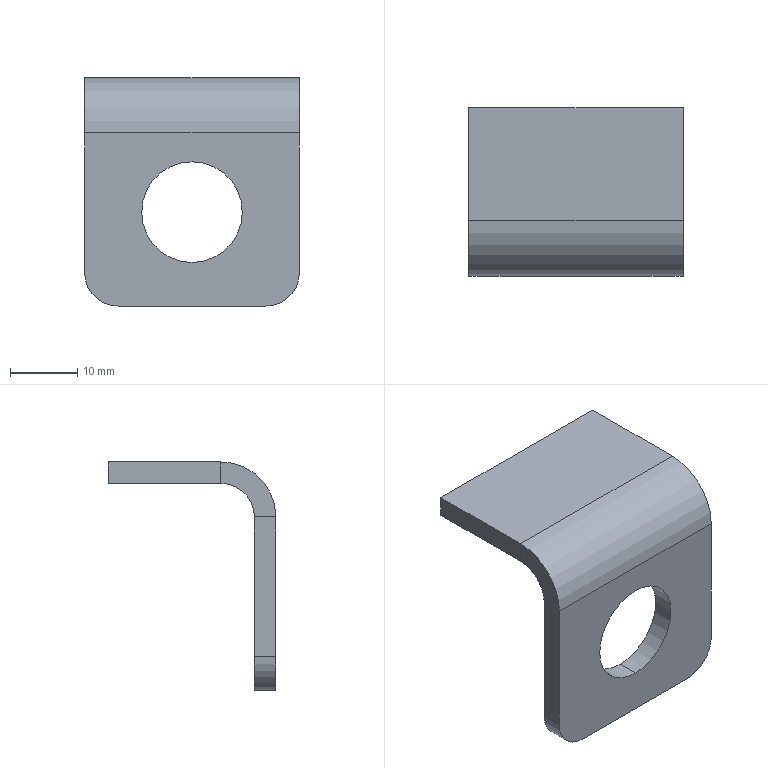Part | SolidWorks | features Fillet 1, FlatPattern 1, ICE 1, SMBaseFlange 1, SheetMetal 1 | 1 solid | 18 faces | box 32 x 25 x 34 mm | volume 4824 mm3 | plane 12 | cylinder 6 | commonest cylinder face diameters 10 x3 15 x2 16.4 x1
STEP:
#1=CARTESIAN_POINT('',(0.,3.2,-12.5));
#2=VERTEX_POINT('',#1);
#3=CARTESIAN_POINT('',(0.,3.2,-27.5));
#4=VERTEX_POINT('',#3);
#5=CARTESIAN_POINT('',(0.,3.2,-20.));
#6=DIRECTION('',(0.,-1.,0.));
#7=DIRECTION('',(0.,0.,-1.));
#8=AXIS2_PLACEMENT_3D('',#5,#6,#7);
#9=CIRCLE('',#8,7.5);
#10=EDGE_CURVE('',#2,#4,#9,.T.);
#11=ORIENTED_EDGE('',*,*,#10,.F.);
#12=CARTESIAN_POINT('',(0.,0.,-12.5));
#13=VERTEX_POINT('',#12);
#14=CARTESIAN_POINT('',(0.,25.,-12.5));
#15=DIRECTION('',(0.,-1.,0.));
#16=VECTOR('',#15,1000.);
#17=LINE('',#14,#16);
#18=EDGE_CURVE('',#2,#13,#17,.T.);
#19=ORIENTED_EDGE('',*,*,#18,.T.);
#20=CARTESIAN_POINT('',(0.,0.,-27.5));
#21=VERTEX_POINT('',#20);
#22=CARTESIAN_POINT('',(0.,0.,-20.));
#23=DIRECTION('',(0.,-1.,0.));
#24=DIRECTION('',(0.,0.,-1.));
#25=AXIS2_PLACEMENT_3D('',#22,#23,#24);
#26=CIRCLE('',#25,7.5);
#27=EDGE_CURVE('',#13,#21,#26,.T.);
#28=ORIENTED_EDGE('',*,*,#27,.T.);
#29=CARTESIAN_POINT('',(0.,25.,-27.5));
#30=DIRECTION('',(0.,-1.,0.));
#31=VECTOR('',#30,1000.);
#32=LINE('',#29,#31);
#33=EDGE_CURVE('',#4,#21,#32,.T.);
#34=ORIENTED_EDGE('',*,*,#33,.F.);
#35=EDGE_LOOP('',(#11,#19,#28,#34));
#36=FACE_OUTER_BOUND('',#35,.T.);
#37=CARTESIAN_POINT('',(0.,25.,-20.));
#38=DIRECTION('',(0.,-1.,0.));
#39=DIRECTION('',(0.,0.,-1.));
#40=AXIS2_PLACEMENT_3D('',#37,#38,#39);
#41=CYLINDRICAL_SURFACE('',#40,7.5);
#42=ADVANCED_FACE('',(#36),#41,.F.);
#43=CARTESIAN_POINT('',(16.,8.2,0.));
#44=VERTEX_POINT('',#43);
#45=CARTESIAN_POINT('',(16.,8.2,-3.2));
#46=VERTEX_POINT('',#45);
#47=CARTESIAN_POINT('',(16.,8.2,0.));
#48=DIRECTION('',(0.,0.,-1.));
#49=VECTOR('',#48,1000.);
#50=LINE('',#47,#49);
#51=EDGE_CURVE('',#44,#46,#50,.T.);
#52=ORIENTED_EDGE('',*,*,#51,.F.);
#53=CARTESIAN_POINT('',(16.,0.,-8.2));
#54=VERTEX_POINT('',#53);
#55=CARTESIAN_POINT('',(16.,8.2,-8.2));
#56=DIRECTION('',(-1.,0.,0.));
#57=DIRECTION('',(0.,0.,-1.));
#58=AXIS2_PLACEMENT_3D('',#55,#56,#57);
#59=CIRCLE('',#58,8.2);
#60=EDGE_CURVE('',#54,#44,#59,.T.);
#61=ORIENTED_EDGE('',*,*,#60,.F.);
#62=CARTESIAN_POINT('',(16.,3.2,-8.2));
#63=VERTEX_POINT('',#62);
#64=CARTESIAN_POINT('',(16.,3.2,-8.2));
#65=DIRECTION('',(0.,-1.,0.));
#66=VECTOR('',#65,1000.);
#67=LINE('',#64,#66);
#68=EDGE_CURVE('',#63,#54,#67,.T.);
#69=ORIENTED_EDGE('',*,*,#68,.F.);
#70=CARTESIAN_POINT('',(16.,8.2,-8.2));
#71=DIRECTION('',(-1.,0.,0.));
#72=DIRECTION('',(0.,0.,-1.));
#73=AXIS2_PLACEMENT_3D('',#70,#71,#72);
#74=CIRCLE('',#73,5.);
#75=EDGE_CURVE('',#63,#46,#74,.T.);
#76=ORIENTED_EDGE('',*,*,#75,.T.);
#77=EDGE_LOOP('',(#52,#61,#69,#76));
#78=FACE_OUTER_BOUND('',#77,.T.);
#79=CARTESIAN_POINT('',(16.,8.2,0.));
#80=DIRECTION('',(1.,0.,0.));
#81=DIRECTION('',(0.,0.,-1.));
#82=AXIS2_PLACEMENT_3D('',#79,#80,#81);
#83=PLANE('',#82);
#84=ADVANCED_FACE('',(#78),#83,.T.);
#85=CARTESIAN_POINT('',(16.,25.,0.));
#86=VERTEX_POINT('',#85);
#87=CARTESIAN_POINT('',(16.,0.,0.));
#88=DIRECTION('',(0.,1.,0.));
#89=VECTOR('',#88,1000.);
#90=LINE('',#87,#89);
#91=EDGE_CURVE('',#44,#86,#90,.T.);
#92=ORIENTED_EDGE('',*,*,#91,.F.);
#93=ORIENTED_EDGE('',*,*,#51,.T.);
#94=CARTESIAN_POINT('',(16.,25.,-3.2));
#95=VERTEX_POINT('',#94);
#96=CARTESIAN_POINT('',(16.,0.,-3.2));
#97=DIRECTION('',(0.,1.,0.));
#98=VECTOR('',#97,1000.);
#99=LINE('',#96,#98);
#100=EDGE_CURVE('',#46,#95,#99,.T.);
#101=ORIENTED_EDGE('',*,*,#100,.T.);
#102=CARTESIAN_POINT('',(16.,25.,0.));
#103=DIRECTION('',(0.,0.,-1.));
#104=VECTOR('',#103,1000.);
#105=LINE('',#102,#104);
#106=EDGE_CURVE('',#86,#95,#105,.T.);
#107=ORIENTED_EDGE('',*,*,#106,.F.);
#108=EDGE_LOOP('',(#92,#93,#101,#107));
#109=FACE_OUTER_BOUND('',#108,.T.);
#110=CARTESIAN_POINT('',(16.,3.2,-8.2));
#111=DIRECTION('',(1.,0.,0.));
#112=DIRECTION('',(0.,0.,-1.));
#113=AXIS2_PLACEMENT_3D('',#110,#111,#112);
#114=PLANE('',#113);
#115=ADVANCED_FACE('',(#109),#114,.T.);
#116=CARTESIAN_POINT('',(-16.,0.,-8.2));
#117=VERTEX_POINT('',#116);
#118=CARTESIAN_POINT('',(-16.,3.2,-8.2));
#119=VERTEX_POINT('',#118);
#120=CARTESIAN_POINT('',(-16.,0.,-8.2));
#121=DIRECTION('',(0.,1.,0.));
#122=VECTOR('',#121,1000.);
#123=LINE('',#120,#122);
#124=EDGE_CURVE('',#117,#119,#123,.T.);
#125=ORIENTED_EDGE('',*,*,#124,.F.);
#126=CARTESIAN_POINT('',(-16.,8.2,0.));
#127=VERTEX_POINT('',#126);
#128=CARTESIAN_POINT('',(-16.,8.2,-8.2));
#129=DIRECTION('',(-1.,0.,0.));
#130=DIRECTION('',(0.,0.,-1.));
#131=AXIS2_PLACEMENT_3D('',#128,#129,#130);
#132=CIRCLE('',#131,8.2);
#133=EDGE_CURVE('',#117,#127,#132,.T.);
#134=ORIENTED_EDGE('',*,*,#133,.T.);
#135=CARTESIAN_POINT('',(-16.,8.2,-3.2));
#136=VERTEX_POINT('',#135);
#137=CARTESIAN_POINT('',(-16.,8.2,-3.2));
#138=DIRECTION('',(0.,0.,1.));
#139=VECTOR('',#138,1000.);
#140=LINE('',#137,#139);
#141=EDGE_CURVE('',#136,#127,#140,.T.);
#142=ORIENTED_EDGE('',*,*,#141,.F.);
#143=CARTESIAN_POINT('',(-16.,8.2,-8.2));
#144=DIRECTION('',(-1.,0.,0.));
#145=DIRECTION('',(0.,0.,-1.));
#146=AXIS2_PLACEMENT_3D('',#143,#144,#145);
#147=CIRCLE('',#146,5.);
#148=EDGE_CURVE('',#119,#136,#147,.T.);
#149=ORIENTED_EDGE('',*,*,#148,.F.);
#150=EDGE_LOOP('',(#125,#134,#142,#149));
#151=FACE_OUTER_BOUND('',#150,.T.);
#152=CARTESIAN_POINT('',(-16.,0.,-8.2));
#153=DIRECTION('',(-1.,0.,0.));
#154=DIRECTION('',(0.,0.,1.));
#155=AXIS2_PLACEMENT_3D('',#152,#153,#154);
#156=PLANE('',#155);
#157=ADVANCED_FACE('',(#151),#156,.T.);
#158=CARTESIAN_POINT('',(-16.,3.2,-29.));
#159=VERTEX_POINT('',#158);
#160=CARTESIAN_POINT('',(-16.,3.2,0.));
#161=DIRECTION('',(0.,0.,1.));
#162=VECTOR('',#161,1000.);
#163=LINE('',#160,#162);
#164=EDGE_CURVE('',#159,#119,#163,.T.);
#165=ORIENTED_EDGE('',*,*,#164,.F.);
#166=CARTESIAN_POINT('',(-16.,0.,-29.));
#167=VERTEX_POINT('',#166);
#168=CARTESIAN_POINT('',(-16.,8.2,-29.));
#169=DIRECTION('',(0.,-1.,0.));
#170=VECTOR('',#169,1000.);
#171=LINE('',#168,#170);
#172=EDGE_CURVE('',#159,#167,#171,.T.);
#173=ORIENTED_EDGE('',*,*,#172,.T.);
#174=CARTESIAN_POINT('',(-16.,0.,0.));
#175=DIRECTION('',(0.,0.,1.));
#176=VECTOR('',#175,1000.);
#177=LINE('',#174,#176);
#178=EDGE_CURVE('',#167,#117,#177,.T.);
#179=ORIENTED_EDGE('',*,*,#178,.T.);
#180=ORIENTED_EDGE('',*,*,#124,.T.);
#181=EDGE_LOOP('',(#165,#173,#179,#180));
#182=FACE_OUTER_BOUND('',#181,.T.);
#183=CARTESIAN_POINT('',(-16.,8.2,-3.2));
#184=DIRECTION('',(-1.,0.,0.));
#185=DIRECTION('',(0.,0.,1.));
#186=AXIS2_PLACEMENT_3D('',#183,#184,#185);
#187=PLANE('',#186);
#188=ADVANCED_FACE('',(#182),#187,.T.);
#189=CARTESIAN_POINT('',(-16.,25.,-3.2));
#190=VERTEX_POINT('',#189);
#191=CARTESIAN_POINT('',(-16.,0.,-3.2));
#192=DIRECTION('',(0.,1.,0.));
#193=VECTOR('',#192,1000.);
#194=LINE('',#191,#193);
#195=EDGE_CURVE('',#136,#190,#194,.T.);
#196=ORIENTED_EDGE('',*,*,#195,.T.);
#197=CARTESIAN_POINT('',(16.,25.,-3.2));
#198=DIRECTION('',(-1.,0.,0.));
#199=VECTOR('',#198,1000.);
#200=LINE('',#197,#199);
#201=EDGE_CURVE('',#95,#190,#200,.T.);
#202=ORIENTED_EDGE('',*,*,#201,.F.);
#203=ORIENTED_EDGE('',*,*,#100,.F.);
#204=CARTESIAN_POINT('',(16.,8.2,-3.2));
#205=DIRECTION('',(-1.,0.,0.));
#206=VECTOR('',#205,1000.);
#207=LINE('',#204,#206);
#208=EDGE_CURVE('',#46,#136,#207,.T.);
#209=ORIENTED_EDGE('',*,*,#208,.T.);
#210=EDGE_LOOP('',(#196,#202,#203,#209));
#211=FACE_OUTER_BOUND('',#210,.T.);
#212=CARTESIAN_POINT('',(16.,0.,-3.2));
#213=DIRECTION('',(0.,0.,1.));
#214=DIRECTION('',(1.,0.,0.));
#215=AXIS2_PLACEMENT_3D('',#212,#213,#214);
#216=PLANE('',#215);
#217=ADVANCED_FACE('',(#211),#216,.F.);
#218=CARTESIAN_POINT('',(-16.,25.,0.));
#219=VERTEX_POINT('',#218);
#220=CARTESIAN_POINT('',(-16.,25.,0.));
#221=DIRECTION('',(0.,0.,-1.));
#222=VECTOR('',#221,1000.);
#223=LINE('',#220,#222);
#224=EDGE_CURVE('',#219,#190,#223,.T.);
#225=ORIENTED_EDGE('',*,*,#224,.F.);
#226=CARTESIAN_POINT('',(16.,25.,0.));
#227=DIRECTION('',(-1.,0.,0.));
#228=VECTOR('',#227,1000.);
#229=LINE('',#226,#228);
#230=EDGE_CURVE('',#86,#219,#229,.T.);
#231=ORIENTED_EDGE('',*,*,#230,.F.);
#232=ORIENTED_EDGE('',*,*,#106,.T.);
#233=ORIENTED_EDGE('',*,*,#201,.T.);
#234=EDGE_LOOP('',(#225,#231,#232,#233));
#235=FACE_OUTER_BOUND('',#234,.T.);
#236=CARTESIAN_POINT('',(16.,25.,0.));
#237=DIRECTION('',(0.,1.,0.));
#238=DIRECTION('',(0.,0.,1.));
#239=AXIS2_PLACEMENT_3D('',#236,#237,#238);
#240=PLANE('',#239);
#241=ADVANCED_FACE('',(#235),#240,.T.);
#242=CARTESIAN_POINT('',(-16.,0.,0.));
#243=DIRECTION('',(0.,1.,0.));
#244=VECTOR('',#243,1000.);
#245=LINE('',#242,#244);
#246=EDGE_CURVE('',#127,#219,#245,.T.);
#247=ORIENTED_EDGE('',*,*,#246,.F.);
#248=CARTESIAN_POINT('',(16.,8.2,0.));
#249=DIRECTION('',(-1.,0.,0.));
#250=VECTOR('',#249,1000.);
#251=LINE('',#248,#250);
#252=EDGE_CURVE('',#44,#127,#251,.T.);
#253=ORIENTED_EDGE('',*,*,#252,.F.);
#254=ORIENTED_EDGE('',*,*,#91,.T.);
#255=ORIENTED_EDGE('',*,*,#230,.T.);
#256=EDGE_LOOP('',(#247,#253,#254,#255));
#257=FACE_OUTER_BOUND('',#256,.T.);
#258=CARTESIAN_POINT('',(16.,0.,0.));
#259=DIRECTION('',(0.,0.,1.));
#260=DIRECTION('',(1.,0.,0.));
#261=AXIS2_PLACEMENT_3D('',#258,#259,#260);
#262=PLANE('',#261);
#263=ADVANCED_FACE('',(#257),#262,.T.);
#264=ORIENTED_EDGE('',*,*,#133,.F.);
#265=CARTESIAN_POINT('',(16.,0.,-8.2));
#266=DIRECTION('',(-1.,0.,0.));
#267=VECTOR('',#266,1000.);
#268=LINE('',#265,#267);
#269=EDGE_CURVE('',#54,#117,#268,.T.);
#270=ORIENTED_EDGE('',*,*,#269,.F.);
#271=ORIENTED_EDGE('',*,*,#60,.T.);
#272=ORIENTED_EDGE('',*,*,#252,.T.);
#273=EDGE_LOOP('',(#264,#270,#271,#272));
#274=FACE_OUTER_BOUND('',#273,.T.);
#275=CARTESIAN_POINT('',(16.,8.2,-8.2));
#276=DIRECTION('',(-1.,0.,0.));
#277=DIRECTION('',(0.,0.,1.));
#278=AXIS2_PLACEMENT_3D('',#275,#276,#277);
#279=CYLINDRICAL_SURFACE('',#278,8.2);
#280=ADVANCED_FACE('',(#274),#279,.T.);
#281=CARTESIAN_POINT('',(0.,0.,-20.));
#282=DIRECTION('',(0.,-1.,0.));
#283=DIRECTION('',(0.,0.,-1.));
#284=AXIS2_PLACEMENT_3D('',#281,#282,#283);
#285=CIRCLE('',#284,7.5);
#286=EDGE_CURVE('',#21,#13,#285,.T.);
#287=ORIENTED_EDGE('',*,*,#286,.F.);
#288=ORIENTED_EDGE('',*,*,#27,.F.);
#289=EDGE_LOOP('',(#287,#288));
#290=FACE_BOUND('',#289,.T.);
#291=ORIENTED_EDGE('',*,*,#178,.F.);
#292=CARTESIAN_POINT('',(-11.,0.,-34.));
#293=VERTEX_POINT('',#292);
#294=CARTESIAN_POINT('',(-11.,0.,-29.));
#295=DIRECTION('',(0.,-1.,0.));
#296=DIRECTION('',(0.,0.,-1.));
#297=AXIS2_PLACEMENT_3D('',#294,#295,#296);
#298=CIRCLE('',#297,5.);
#299=EDGE_CURVE('',#167,#293,#298,.T.);
#300=ORIENTED_EDGE('',*,*,#299,.T.);
#301=CARTESIAN_POINT('',(11.,0.,-34.));
#302=VERTEX_POINT('',#301);
#303=CARTESIAN_POINT('',(16.,0.,-34.));
#304=DIRECTION('',(-1.,0.,0.));
#305=VECTOR('',#304,1000.);
#306=LINE('',#303,#305);
#307=EDGE_CURVE('',#302,#293,#306,.T.);
#308=ORIENTED_EDGE('',*,*,#307,.F.);
#309=CARTESIAN_POINT('',(16.,0.,-29.));
#310=VERTEX_POINT('',#309);
#311=CARTESIAN_POINT('',(11.,0.,-29.));
#312=DIRECTION('',(0.,-1.,0.));
#313=DIRECTION('',(0.,0.,-1.));
#314=AXIS2_PLACEMENT_3D('',#311,#312,#313);
#315=CIRCLE('',#314,5.);
#316=EDGE_CURVE('',#302,#310,#315,.T.);
#317=ORIENTED_EDGE('',*,*,#316,.T.);
#318=CARTESIAN_POINT('',(16.,0.,0.));
#319=DIRECTION('',(0.,0.,1.));
#320=VECTOR('',#319,1000.);
#321=LINE('',#318,#320);
#322=EDGE_CURVE('',#310,#54,#321,.T.);
#323=ORIENTED_EDGE('',*,*,#322,.T.);
#324=ORIENTED_EDGE('',*,*,#269,.T.);
#325=EDGE_LOOP('',(#291,#300,#308,#317,#323,#324));
#326=FACE_OUTER_BOUND('',#325,.T.);
#327=CARTESIAN_POINT('',(16.,0.,0.));
#328=DIRECTION('',(0.,-1.,0.));
#329=DIRECTION('',(0.,0.,-1.));
#330=AXIS2_PLACEMENT_3D('',#327,#328,#329);
#331=PLANE('',#330);
#332=ADVANCED_FACE('',(#290,#326),#331,.T.);
#333=ORIENTED_EDGE('',*,*,#307,.T.);
#334=CARTESIAN_POINT('',(-11.,3.2,-34.));
#335=VERTEX_POINT('',#334);
#336=CARTESIAN_POINT('',(-11.,3.2,-34.));
#337=DIRECTION('',(0.,1.,0.));
#338=VECTOR('',#337,1000.);
#339=LINE('',#336,#338);
#340=EDGE_CURVE('',#293,#335,#339,.T.);
#341=ORIENTED_EDGE('',*,*,#340,.T.);
#342=CARTESIAN_POINT('',(11.,3.2,-34.));
#343=VERTEX_POINT('',#342);
#344=CARTESIAN_POINT('',(16.,3.2,-34.));
#345=DIRECTION('',(-1.,0.,0.));
#346=VECTOR('',#345,1000.);
#347=LINE('',#344,#346);
#348=EDGE_CURVE('',#343,#335,#347,.T.);
#349=ORIENTED_EDGE('',*,*,#348,.F.);
#350=CARTESIAN_POINT('',(11.,3.2,-34.));
#351=DIRECTION('',(0.,-1.,0.));
#352=VECTOR('',#351,1000.);
#353=LINE('',#350,#352);
#354=EDGE_CURVE('',#343,#302,#353,.T.);
#355=ORIENTED_EDGE('',*,*,#354,.T.);
#356=EDGE_LOOP('',(#333,#341,#349,#355));
#357=FACE_OUTER_BOUND('',#356,.T.);
#358=CARTESIAN_POINT('',(16.,3.2,-34.));
#359=DIRECTION('',(0.,0.,-1.));
#360=DIRECTION('',(-1.,0.,0.));
#361=AXIS2_PLACEMENT_3D('',#358,#359,#360);
#362=PLANE('',#361);
#363=ADVANCED_FACE('',(#357),#362,.T.);
#364=CARTESIAN_POINT('',(0.,3.2,-20.));
#365=DIRECTION('',(0.,-1.,0.));
#366=DIRECTION('',(0.,0.,-1.));
#367=AXIS2_PLACEMENT_3D('',#364,#365,#366);
#368=CIRCLE('',#367,7.5);
#369=EDGE_CURVE('',#4,#2,#368,.T.);
#370=ORIENTED_EDGE('',*,*,#369,.T.);
#371=ORIENTED_EDGE('',*,*,#10,.T.);
#372=EDGE_LOOP('',(#370,#371));
#373=FACE_BOUND('',#372,.T.);
#374=ORIENTED_EDGE('',*,*,#348,.T.);
#375=CARTESIAN_POINT('',(-11.,3.2,-29.));
#376=DIRECTION('',(0.,1.,0.));
#377=DIRECTION('',(0.,0.,-1.));
#378=AXIS2_PLACEMENT_3D('',#375,#376,#377);
#379=CIRCLE('',#378,5.);
#380=EDGE_CURVE('',#335,#159,#379,.T.);
#381=ORIENTED_EDGE('',*,*,#380,.T.);
#382=ORIENTED_EDGE('',*,*,#164,.T.);
#383=CARTESIAN_POINT('',(16.,3.2,-8.2));
#384=DIRECTION('',(-1.,0.,0.));
#385=VECTOR('',#384,1000.);
#386=LINE('',#383,#385);
#387=EDGE_CURVE('',#63,#119,#386,.T.);
#388=ORIENTED_EDGE('',*,*,#387,.F.);
#389=CARTESIAN_POINT('',(16.,3.2,-29.));
#390=VERTEX_POINT('',#389);
#391=CARTESIAN_POINT('',(16.,3.2,0.));
#392=DIRECTION('',(0.,0.,1.));
#393=VECTOR('',#392,1000.);
#394=LINE('',#391,#393);
#395=EDGE_CURVE('',#390,#63,#394,.T.);
#396=ORIENTED_EDGE('',*,*,#395,.F.);
#397=CARTESIAN_POINT('',(11.,3.2,-29.));
#398=DIRECTION('',(0.,1.,0.));
#399=DIRECTION('',(0.,0.,-1.));
#400=AXIS2_PLACEMENT_3D('',#397,#398,#399);
#401=CIRCLE('',#400,5.);
#402=EDGE_CURVE('',#390,#343,#401,.T.);
#403=ORIENTED_EDGE('',*,*,#402,.T.);
#404=EDGE_LOOP('',(#374,#381,#382,#388,#396,#403));
#405=FACE_OUTER_BOUND('',#404,.T.);
#406=CARTESIAN_POINT('',(16.,3.2,0.));
#407=DIRECTION('',(0.,-1.,0.));
#408=DIRECTION('',(0.,0.,-1.));
#409=AXIS2_PLACEMENT_3D('',#406,#407,#408);
#410=PLANE('',#409);
#411=ADVANCED_FACE('',(#373,#405),#410,.F.);
#412=ORIENTED_EDGE('',*,*,#148,.T.);
#413=ORIENTED_EDGE('',*,*,#208,.F.);
#414=ORIENTED_EDGE('',*,*,#75,.F.);
#415=ORIENTED_EDGE('',*,*,#387,.T.);
#416=EDGE_LOOP('',(#412,#413,#414,#415));
#417=FACE_OUTER_BOUND('',#416,.T.);
#418=CARTESIAN_POINT('',(16.,8.2,-8.2));
#419=DIRECTION('',(-1.,0.,0.));
#420=DIRECTION('',(0.,0.,1.));
#421=AXIS2_PLACEMENT_3D('',#418,#419,#420);
#422=CYLINDRICAL_SURFACE('',#421,5.);
#423=ADVANCED_FACE('',(#417),#422,.F.);
#424=ORIENTED_EDGE('',*,*,#322,.F.);
#425=CARTESIAN_POINT('',(16.,8.2,-29.));
#426=DIRECTION('',(0.,1.,0.));
#427=VECTOR('',#426,1000.);
#428=LINE('',#425,#427);
#429=EDGE_CURVE('',#310,#390,#428,.T.);
#430=ORIENTED_EDGE('',*,*,#429,.T.);
#431=ORIENTED_EDGE('',*,*,#395,.T.);
#432=ORIENTED_EDGE('',*,*,#68,.T.);
#433=EDGE_LOOP('',(#424,#430,#431,#432));
#434=FACE_OUTER_BOUND('',#433,.T.);
#435=CARTESIAN_POINT('',(16.,8.2,-8.2));
#436=DIRECTION('',(1.,0.,0.));
#437=DIRECTION('',(0.,0.,-1.));
#438=AXIS2_PLACEMENT_3D('',#435,#436,#437);
#439=PLANE('',#438);
#440=ADVANCED_FACE('',(#434),#439,.T.);
#441=ORIENTED_EDGE('',*,*,#195,.F.);
#442=ORIENTED_EDGE('',*,*,#141,.T.);
#443=ORIENTED_EDGE('',*,*,#246,.T.);
#444=ORIENTED_EDGE('',*,*,#224,.T.);
#445=EDGE_LOOP('',(#441,#442,#443,#444));
#446=FACE_OUTER_BOUND('',#445,.T.);
#447=CARTESIAN_POINT('',(-16.,8.2,-8.2));
#448=DIRECTION('',(1.,0.,0.));
#449=DIRECTION('',(0.,0.,-1.));
#450=AXIS2_PLACEMENT_3D('',#447,#448,#449);
#451=PLANE('',#450);
#452=ADVANCED_FACE('',(#446),#451,.F.);
#453=ORIENTED_EDGE('',*,*,#18,.F.);
#454=ORIENTED_EDGE('',*,*,#369,.F.);
#455=ORIENTED_EDGE('',*,*,#33,.T.);
#456=ORIENTED_EDGE('',*,*,#286,.T.);
#457=EDGE_LOOP('',(#453,#454,#455,#456));
#458=FACE_OUTER_BOUND('',#457,.T.);
#459=CARTESIAN_POINT('',(0.,25.,-20.));
#460=DIRECTION('',(0.,-1.,0.));
#461=DIRECTION('',(0.,0.,-1.));
#462=AXIS2_PLACEMENT_3D('',#459,#460,#461);
#463=CYLINDRICAL_SURFACE('',#462,7.5);
#464=ADVANCED_FACE('',(#458),#463,.F.);
#465=ORIENTED_EDGE('',*,*,#380,.F.);
#466=ORIENTED_EDGE('',*,*,#340,.F.);
#467=ORIENTED_EDGE('',*,*,#299,.F.);
#468=ORIENTED_EDGE('',*,*,#172,.F.);
#469=EDGE_LOOP('',(#465,#466,#467,#468));
#470=FACE_OUTER_BOUND('',#469,.T.);
#471=CARTESIAN_POINT('',(-11.,8.2,-29.));
#472=DIRECTION('',(0.,-1.,0.));
#473=DIRECTION('',(0.,0.,-1.));
#474=AXIS2_PLACEMENT_3D('',#471,#472,#473);
#475=CYLINDRICAL_SURFACE('',#474,5.);
#476=ADVANCED_FACE('',(#470),#475,.T.);
#477=ORIENTED_EDGE('',*,*,#402,.F.);
#478=ORIENTED_EDGE('',*,*,#429,.F.);
#479=ORIENTED_EDGE('',*,*,#316,.F.);
#480=ORIENTED_EDGE('',*,*,#354,.F.);
#481=EDGE_LOOP('',(#477,#478,#479,#480));
#482=FACE_OUTER_BOUND('',#481,.T.);
#483=CARTESIAN_POINT('',(11.,3.2,-29.));
#484=DIRECTION('',(0.,-1.,0.));
#485=DIRECTION('',(0.,0.,-1.));
#486=AXIS2_PLACEMENT_3D('',#483,#484,#485);
#487=CYLINDRICAL_SURFACE('',#486,5.);
#488=ADVANCED_FACE('',(#482),#487,.T.);
#489=CLOSED_SHELL('',(#42,#84,#115,#157,#188,#217,#241,#263,#280,#332,#363,#411,#423,#440,#452,#464,#476,#488));
#490=MANIFOLD_SOLID_BREP('',#489);
#491=CARTESIAN_POINT('',(0.,0.,0.));
#492=DIRECTION('',(0.,0.,1.));
#493=DIRECTION('',(1.,0.,0.));
#494=AXIS2_PLACEMENT_3D('',#491,#492,#493);
#495=(LENGTH_UNIT()NAMED_UNIT(*)SI_UNIT(.MILLI.,.METRE.));
#496=UNCERTAINTY_MEASURE_WITH_UNIT(LENGTH_MEASURE(0.00001),#495,'','');
#497=(NAMED_UNIT(*)PLANE_ANGLE_UNIT()SI_UNIT($,.RADIAN.));
#498=(NAMED_UNIT(*)SI_UNIT($,.STERADIAN.)SOLID_ANGLE_UNIT());
#499=(GEOMETRIC_REPRESENTATION_CONTEXT(3)GLOBAL_UNCERTAINTY_ASSIGNED_CONTEXT((#496))GLOBAL_UNIT_ASSIGNED_CONTEXT((#495,#497,#498))REPRESENTATION_CONTEXT('',''));
#500=ADVANCED_BREP_SHAPE_REPRESENTATION('',(#490,#494),#499);